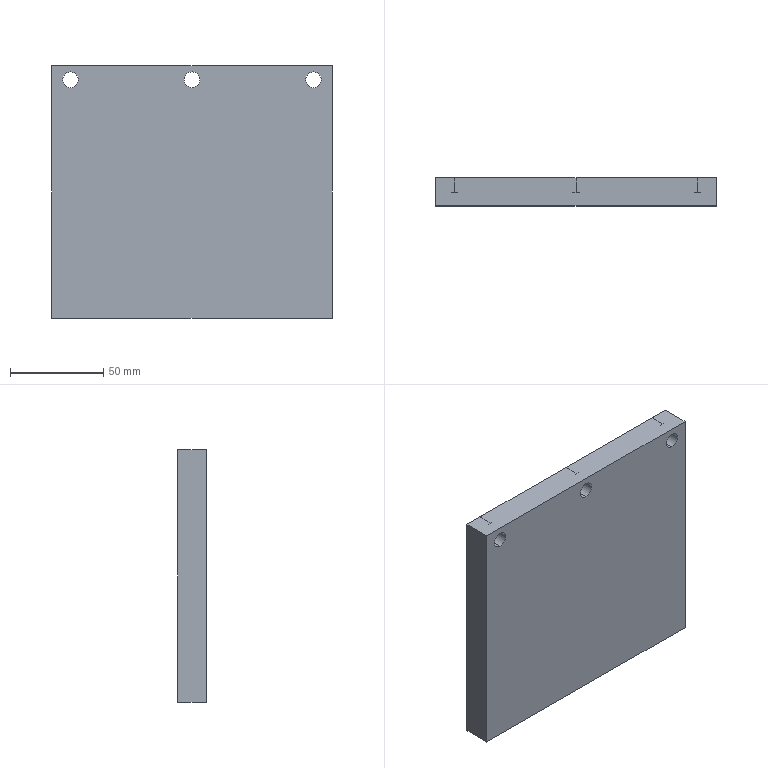Part | STEP file | CON-021 | 1 solid | 21 faces | box 150 x 15 x 135 mm | volume 298623 mm3 | cylinder 12 | plane 9 | commonest cylinder face diameters 8.4 x6 14.5 x6